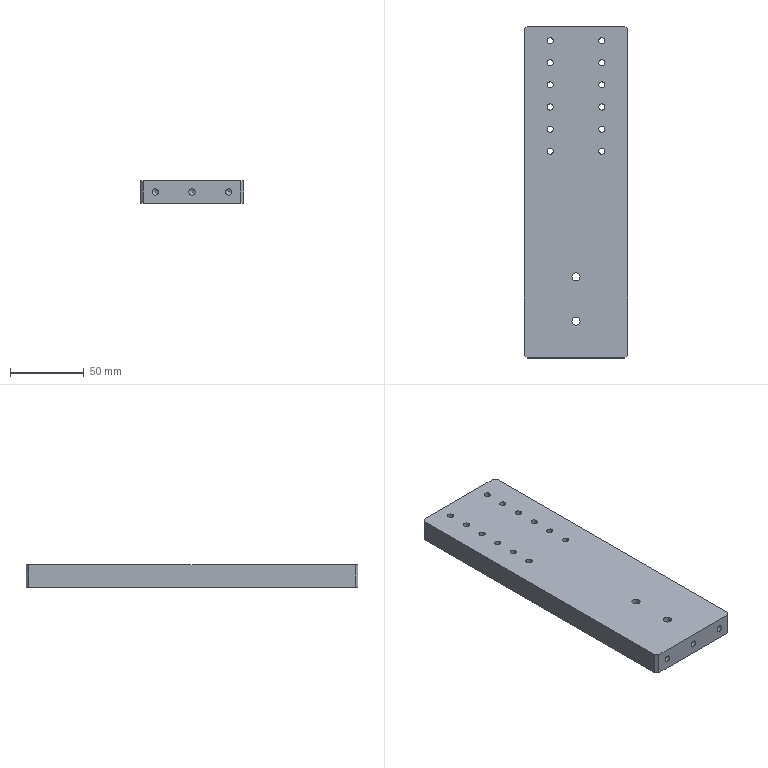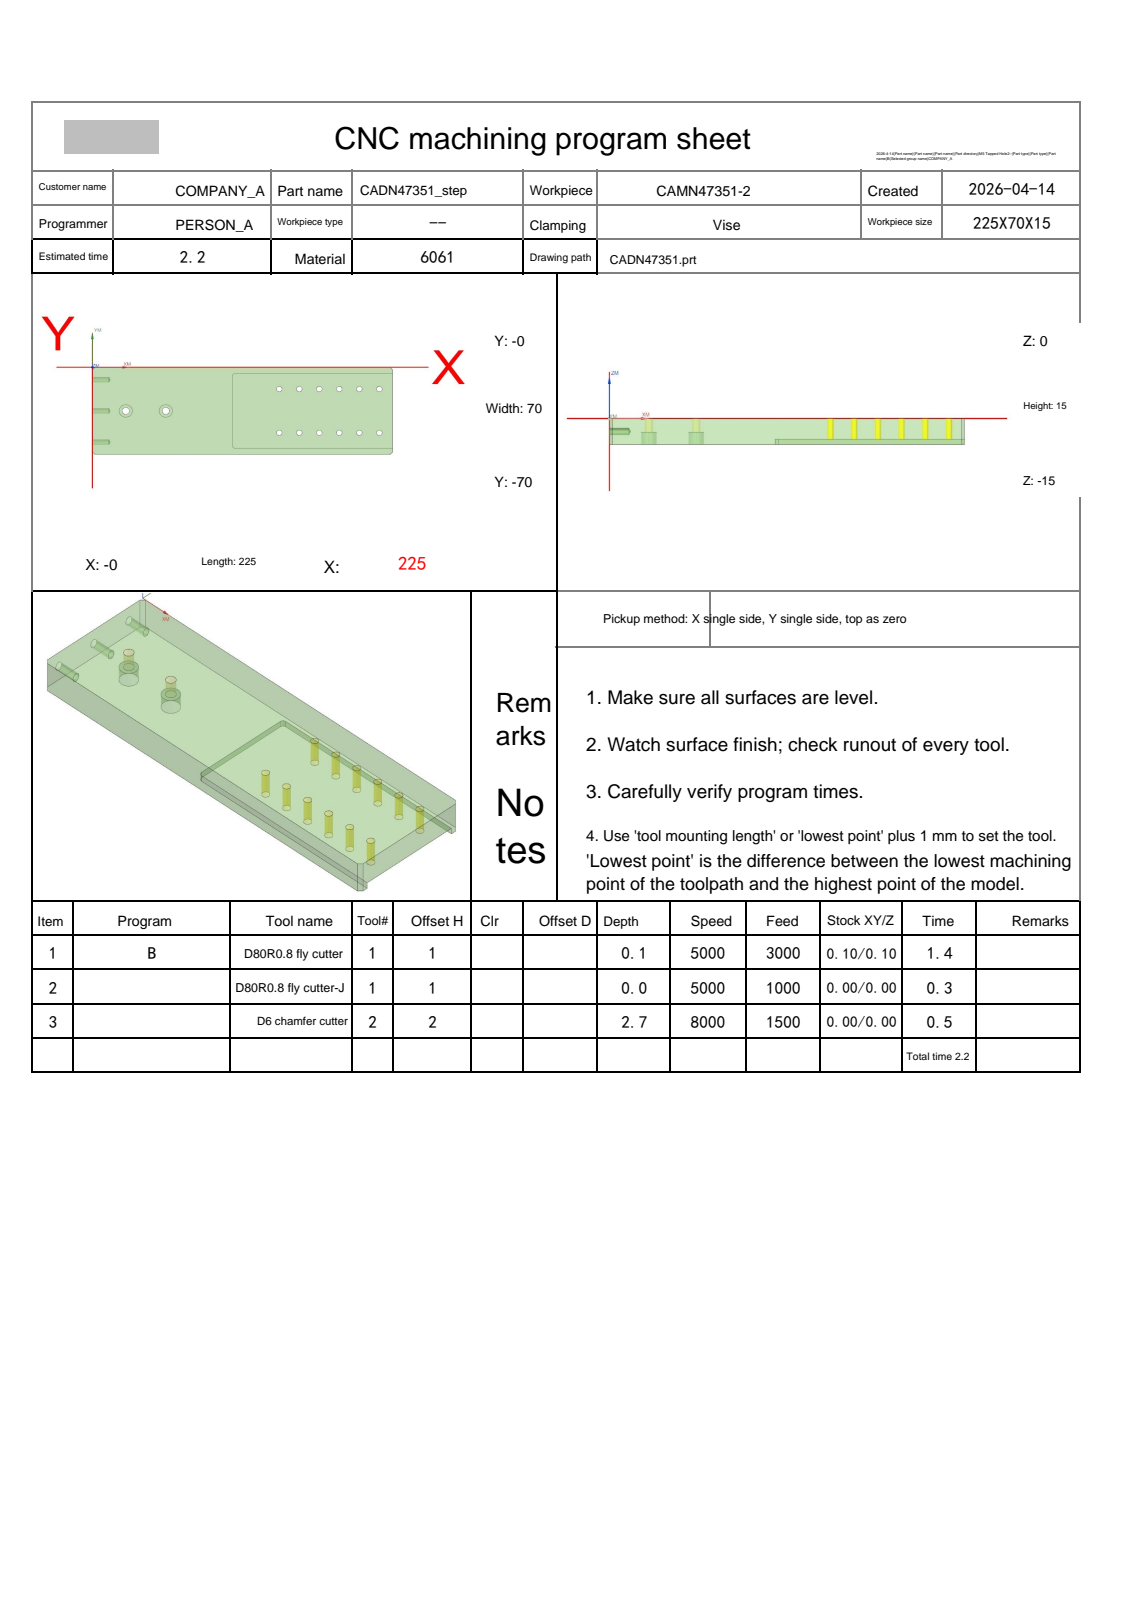NC program | NX | posted by the shop | part box 70 x 225 x 15 mm
Whole program:
%
O0001
(Machine time: 2.81 MIN)
(===Total Tool:2===)
(T1=D80R0.8 fly cutter D=80.  R=0.8  D-  H01 Z=-0.   )
(T2=D6 chamfer cutter   D=6.   R=0.   D-  H02 Z=-2.7  )
G80 G90 G17 G49 G40
G91 G28 Z0
M01
N1 T01 M06
(D80R0.8 fly cutter  D=80. R=0.8 H=01 ce=0.10 di=0.10)
G00 G90 G54 X-52.097 Y-35. M03 S5000
G43 H01 Z20.
M08
Z6.33
G01 Z4.33 F3000.
X-40.097
X265.097
X277.097
Z6.33
G00 X-52.097
Z5.86
G01 Z3.86
X-40.097
X265.097
X277.097
Z5.86
G00 X-52.097
Z5.39
G01 Z3.39
X-40.097
X265.097
X277.097
Z5.39
G00 X-52.097
Z4.92
G01 Z2.92
X-40.097
X265.097
X277.097
Z4.92
G00 Z20.
X-52.097
Z4.45
G01 Z2.45
X-40.097
X265.097
X277.097
Z4.45
G00 Z20.
X-52.097
Z3.98
G01 Z1.98
X-40.097
X265.097
X277.097
Z3.98
G00 Z20.
X-52.097
Z3.51
G01 Z1.51
X-40.097
X265.097
X277.097
Z3.51
G00 Z20.
X-52.097
Z3.04
G01 Z1.04
X-40.097
X265.097
X277.097
Z3.04
G00 Z20.
X-52.097
Z2.57
G01 Z.57
X-40.097
X265.097
X277.097
Z2.57
G00 Z20.
X-52.097
Z2.1
G01 Z.1
X-40.097
X265.097
X277.097
Z2.1
G00 Z20.
G91 G28 Z0.0
M05
M09
G91 G28 Z0.0
M01
N2 T01 M06
(D80R0.8 fly cutter-J  D=80. R=0.8 H=01 ce=0.00 di=0.00)
G00 G90 G54 X-51.999 Y-35. M03 S5000
G43 H01 Z20.
M08
Z2.
G01 Z0.0 F1000.
X-39.999
X264.999
X276.999
Z2.
G00 Z20.
G91 G28 Z0.0
M05
M09
G91 G28 Z0.0
M01
N3 T02 M06
(D6 chamfer cutter  D=6. R=0. H=02 ce=0.00 di=0.00)
G00 G90 G54 X215.071 Y-52.5 M03 S8000
G43 H02 Z20.
M08
G98 G81 X215.071 Y-52.5 Z-2.7 R3. F1000.
X200.071
X185.071
X170.071
X155.071
X140.071
Y-17.5
X155.071
X170.071
X185.071
X200.071
X215.071
G80
G00 Z20.
G00 G90 X112.114 Y1.227 M03 S6500
Z20.
Z.172
G01 Z-1.2 F1500.
G03 X112.4 Y1.027 I1.286 J1.532
G01 X112.446 Y.997
X112.5 Y1.
X223.
X223.259 Y.966
X223.5 Y.866
X223.707 Y.707
X225.707 Y-1.293
X225.866 Y-1.5
X225.966 Y-1.741
X226. Y-2.
Y-68.
X225.966 Y-68.259
X225.866 Y-68.5
X225.707 Y-68.707
X223.707 Y-70.707
X223.5 Y-70.866
X223.259 Y-70.966
X223. Y-71.
X2.
X1.741 Y-70.966
X1.5 Y-70.866
X1.293 Y-70.707
X-.707 Y-68.707
X-.866 Y-68.5
X-.966 Y-68.259
X-1. Y-68.
Y-2.
X-.966 Y-1.741
X-.866 Y-1.5
X-.707 Y-1.293
X1.293 Y.707
X1.5 Y.866
X1.741 Y.966
X2. Y1.
X112.5
X112.554 Y.997
X112.6 Y1.027
G03 X112.886 Y1.227 I-1. J1.732
G01 Z.172
G00 Z10.
X24.593 Y-36.565
Z.27
G01 Z-1.2
G03 X24.898 Y-36.734 I1.118 J1.658
G01 X24.946 Y-36.759
X25. Y-36.75
G03 X26.75 Y-35. I0.0 J1.75
X25. Y-33.25 I-1.75 J0.0
X23.25 Y-35. I0.0 J-1.75
X25. Y-36.75 I1.75 J0.0
G01 X25.054 Y-36.759
X25.102 Y-36.734
G03 X25.407 Y-36.565 I-.813 J1.827
G01 Z.27
G00 Z10.
X54.593
Z.27
G01 Z-1.2
G03 X54.898 Y-36.734 I1.118 J1.658
G01 X54.946 Y-36.759
X55. Y-36.75
G03 X56.75 Y-35. I0.0 J1.75
X55. Y-33.25 I-1.75 J0.0
X53.25 Y-35. I0.0 J-1.75
X55. Y-36.75 I1.75 J0.0
G01 X55.054 Y-36.759
X55.102 Y-36.734
G03 X55.407 Y-36.565 I-.813 J1.827
G01 Z.27
G00 Z20.
M05
M09
G91 G28 Z0.0
G91 G28 Y0.0
M30
%